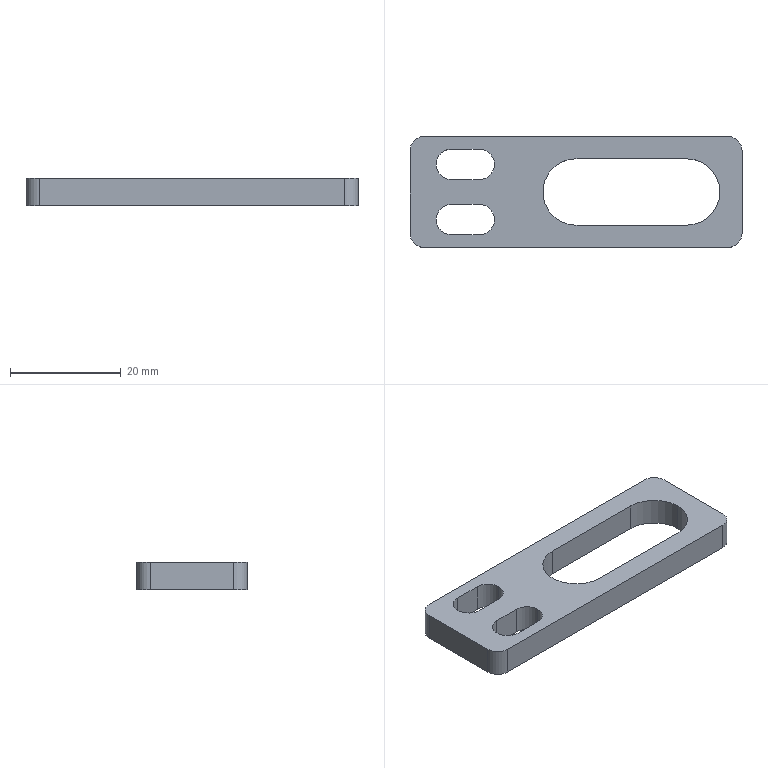Part | STEP file | KF-2212-050-005 | 1 solid | 25 faces | box 60 x 20 x 5 mm | volume 3695 mm3 | cylinder 13 | plane 12 | commonest cylinder face diameters 5.5 x6 5 x4 12 x3
STEP:
#1=CARTESIAN_POINT('',(-14.75,5.,-5.));
#2=VERTEX_POINT('',#1);
#3=CARTESIAN_POINT('',(-17.5,7.75,-5.));
#4=VERTEX_POINT('',#3);
#5=CARTESIAN_POINT('',(-17.5,5.,-5.));
#6=DIRECTION('',(0.,0.,1.));
#7=DIRECTION('',(1.,0.,0.));
#8=AXIS2_PLACEMENT_3D('',#5,#6,#7);
#9=CIRCLE('',#8,2.75);
#10=EDGE_CURVE('',#2,#4,#9,.T.);
#11=ORIENTED_EDGE('',*,*,#10,.F.);
#12=CARTESIAN_POINT('',(-14.75,5.,0.));
#13=VERTEX_POINT('',#12);
#14=CARTESIAN_POINT('',(-14.75,5.,-10.));
#15=DIRECTION('',(0.,0.,1.));
#16=VECTOR('',#15,1000.);
#17=LINE('',#14,#16);
#18=EDGE_CURVE('',#2,#13,#17,.T.);
#19=ORIENTED_EDGE('',*,*,#18,.T.);
#20=CARTESIAN_POINT('',(-17.5,7.75,0.));
#21=VERTEX_POINT('',#20);
#22=CARTESIAN_POINT('',(-17.5,5.,0.));
#23=DIRECTION('',(0.,0.,1.));
#24=DIRECTION('',(1.,0.,0.));
#25=AXIS2_PLACEMENT_3D('',#22,#23,#24);
#26=CIRCLE('',#25,2.75);
#27=EDGE_CURVE('',#13,#21,#26,.T.);
#28=ORIENTED_EDGE('',*,*,#27,.T.);
#29=CARTESIAN_POINT('',(-17.5,7.75,-10.));
#30=DIRECTION('',(0.,0.,1.));
#31=VECTOR('',#30,1000.);
#32=LINE('',#29,#31);
#33=EDGE_CURVE('',#4,#21,#32,.T.);
#34=ORIENTED_EDGE('',*,*,#33,.F.);
#35=EDGE_LOOP('',(#11,#19,#28,#34));
#36=FACE_OUTER_BOUND('',#35,.T.);
#37=CARTESIAN_POINT('',(-17.5,5.,-10.));
#38=DIRECTION('',(0.,0.,1.));
#39=DIRECTION('',(1.,0.,0.));
#40=AXIS2_PLACEMENT_3D('',#37,#38,#39);
#41=CYLINDRICAL_SURFACE('',#40,2.75);
#42=ADVANCED_FACE('',(#36),#41,.F.);
#43=CARTESIAN_POINT('',(-14.75,-5.,-5.));
#44=VERTEX_POINT('',#43);
#45=CARTESIAN_POINT('',(-17.5,-2.25,-5.));
#46=VERTEX_POINT('',#45);
#47=CARTESIAN_POINT('',(-17.5,-5.,-5.));
#48=DIRECTION('',(0.,0.,1.));
#49=DIRECTION('',(1.,0.,0.));
#50=AXIS2_PLACEMENT_3D('',#47,#48,#49);
#51=CIRCLE('',#50,2.75);
#52=EDGE_CURVE('',#44,#46,#51,.T.);
#53=ORIENTED_EDGE('',*,*,#52,.F.);
#54=CARTESIAN_POINT('',(-14.75,-5.,0.));
#55=VERTEX_POINT('',#54);
#56=CARTESIAN_POINT('',(-14.75,-5.,-10.));
#57=DIRECTION('',(0.,0.,1.));
#58=VECTOR('',#57,1000.);
#59=LINE('',#56,#58);
#60=EDGE_CURVE('',#44,#55,#59,.T.);
#61=ORIENTED_EDGE('',*,*,#60,.T.);
#62=CARTESIAN_POINT('',(-17.5,-2.25,0.));
#63=VERTEX_POINT('',#62);
#64=CARTESIAN_POINT('',(-17.5,-5.,0.));
#65=DIRECTION('',(0.,0.,1.));
#66=DIRECTION('',(1.,0.,0.));
#67=AXIS2_PLACEMENT_3D('',#64,#65,#66);
#68=CIRCLE('',#67,2.75);
#69=EDGE_CURVE('',#55,#63,#68,.T.);
#70=ORIENTED_EDGE('',*,*,#69,.T.);
#71=CARTESIAN_POINT('',(-17.5,-2.25,-10.));
#72=DIRECTION('',(0.,0.,1.));
#73=VECTOR('',#72,1000.);
#74=LINE('',#71,#73);
#75=EDGE_CURVE('',#46,#63,#74,.T.);
#76=ORIENTED_EDGE('',*,*,#75,.F.);
#77=EDGE_LOOP('',(#53,#61,#70,#76));
#78=FACE_OUTER_BOUND('',#77,.T.);
#79=CARTESIAN_POINT('',(-17.5,-5.,-10.));
#80=DIRECTION('',(0.,0.,1.));
#81=DIRECTION('',(1.,0.,0.));
#82=AXIS2_PLACEMENT_3D('',#79,#80,#81);
#83=CYLINDRICAL_SURFACE('',#82,2.75);
#84=ADVANCED_FACE('',(#78),#83,.F.);
#85=CARTESIAN_POINT('',(26.,0.,-5.));
#86=VERTEX_POINT('',#85);
#87=CARTESIAN_POINT('',(20.,6.,-5.));
#88=VERTEX_POINT('',#87);
#89=CARTESIAN_POINT('',(20.,0.,-5.));
#90=DIRECTION('',(0.,0.,1.));
#91=DIRECTION('',(1.,0.,0.));
#92=AXIS2_PLACEMENT_3D('',#89,#90,#91);
#93=CIRCLE('',#92,6.);
#94=EDGE_CURVE('',#86,#88,#93,.T.);
#95=ORIENTED_EDGE('',*,*,#94,.F.);
#96=CARTESIAN_POINT('',(26.,0.,0.));
#97=VERTEX_POINT('',#96);
#98=CARTESIAN_POINT('',(26.,0.,-5.));
#99=DIRECTION('',(0.,0.,1.));
#100=VECTOR('',#99,1000.);
#101=LINE('',#98,#100);
#102=EDGE_CURVE('',#86,#97,#101,.T.);
#103=ORIENTED_EDGE('',*,*,#102,.T.);
#104=CARTESIAN_POINT('',(20.,6.,0.));
#105=VERTEX_POINT('',#104);
#106=CARTESIAN_POINT('',(20.,0.,0.));
#107=DIRECTION('',(0.,0.,1.));
#108=DIRECTION('',(1.,0.,0.));
#109=AXIS2_PLACEMENT_3D('',#106,#107,#108);
#110=CIRCLE('',#109,6.);
#111=EDGE_CURVE('',#97,#105,#110,.T.);
#112=ORIENTED_EDGE('',*,*,#111,.T.);
#113=CARTESIAN_POINT('',(20.,6.,-5.));
#114=DIRECTION('',(0.,0.,1.));
#115=VECTOR('',#114,1000.);
#116=LINE('',#113,#115);
#117=EDGE_CURVE('',#88,#105,#116,.T.);
#118=ORIENTED_EDGE('',*,*,#117,.F.);
#119=EDGE_LOOP('',(#95,#103,#112,#118));
#120=FACE_OUTER_BOUND('',#119,.T.);
#121=CARTESIAN_POINT('',(20.,0.,-5.));
#122=DIRECTION('',(0.,0.,1.));
#123=DIRECTION('',(1.,0.,0.));
#124=AXIS2_PLACEMENT_3D('',#121,#122,#123);
#125=CYLINDRICAL_SURFACE('',#124,6.);
#126=ADVANCED_FACE('',(#120),#125,.F.);
#127=CARTESIAN_POINT('',(30.,-7.5,0.));
#128=VERTEX_POINT('',#127);
#129=CARTESIAN_POINT('',(30.,7.5,0.));
#130=VERTEX_POINT('',#129);
#131=CARTESIAN_POINT('',(30.,10.,0.));
#132=DIRECTION('',(0.,1.,0.));
#133=VECTOR('',#132,1000.);
#134=LINE('',#131,#133);
#135=EDGE_CURVE('',#128,#130,#134,.T.);
#136=ORIENTED_EDGE('',*,*,#135,.F.);
#137=CARTESIAN_POINT('',(30.,-7.5,-5.));
#138=VERTEX_POINT('',#137);
#139=CARTESIAN_POINT('',(30.,-7.5,-5.));
#140=DIRECTION('',(0.,0.,-1.));
#141=VECTOR('',#140,1000.);
#142=LINE('',#139,#141);
#143=EDGE_CURVE('',#128,#138,#142,.T.);
#144=ORIENTED_EDGE('',*,*,#143,.T.);
#145=CARTESIAN_POINT('',(30.,7.5,-5.));
#146=VERTEX_POINT('',#145);
#147=CARTESIAN_POINT('',(30.,10.,-5.));
#148=DIRECTION('',(0.,1.,0.));
#149=VECTOR('',#148,1000.);
#150=LINE('',#147,#149);
#151=EDGE_CURVE('',#138,#146,#150,.T.);
#152=ORIENTED_EDGE('',*,*,#151,.T.);
#153=CARTESIAN_POINT('',(30.,7.5,-5.));
#154=DIRECTION('',(0.,0.,1.));
#155=VECTOR('',#154,1000.);
#156=LINE('',#153,#155);
#157=EDGE_CURVE('',#146,#130,#156,.T.);
#158=ORIENTED_EDGE('',*,*,#157,.T.);
#159=EDGE_LOOP('',(#136,#144,#152,#158));
#160=FACE_OUTER_BOUND('',#159,.T.);
#161=CARTESIAN_POINT('',(30.,10.,-5.));
#162=DIRECTION('',(1.,0.,0.));
#163=DIRECTION('',(0.,0.,-1.));
#164=AXIS2_PLACEMENT_3D('',#161,#162,#163);
#165=PLANE('',#164);
#166=ADVANCED_FACE('',(#160),#165,.T.);
#167=CARTESIAN_POINT('',(-27.5,-10.,0.));
#168=VERTEX_POINT('',#167);
#169=CARTESIAN_POINT('',(27.5,-10.,0.));
#170=VERTEX_POINT('',#169);
#171=CARTESIAN_POINT('',(-30.,-10.,0.));
#172=DIRECTION('',(1.,0.,0.));
#173=VECTOR('',#172,1000.);
#174=LINE('',#171,#173);
#175=EDGE_CURVE('',#168,#170,#174,.T.);
#176=ORIENTED_EDGE('',*,*,#175,.F.);
#177=CARTESIAN_POINT('',(-27.5,-10.,-5.));
#178=VERTEX_POINT('',#177);
#179=CARTESIAN_POINT('',(-27.5,-10.,-5.));
#180=DIRECTION('',(0.,0.,-1.));
#181=VECTOR('',#180,1000.);
#182=LINE('',#179,#181);
#183=EDGE_CURVE('',#168,#178,#182,.T.);
#184=ORIENTED_EDGE('',*,*,#183,.T.);
#185=CARTESIAN_POINT('',(27.5,-10.,-5.));
#186=VERTEX_POINT('',#185);
#187=CARTESIAN_POINT('',(-30.,-10.,-5.));
#188=DIRECTION('',(1.,0.,0.));
#189=VECTOR('',#188,1000.);
#190=LINE('',#187,#189);
#191=EDGE_CURVE('',#178,#186,#190,.T.);
#192=ORIENTED_EDGE('',*,*,#191,.T.);
#193=CARTESIAN_POINT('',(27.5,-10.,-5.));
#194=DIRECTION('',(0.,0.,1.));
#195=VECTOR('',#194,1000.);
#196=LINE('',#193,#195);
#197=EDGE_CURVE('',#186,#170,#196,.T.);
#198=ORIENTED_EDGE('',*,*,#197,.T.);
#199=EDGE_LOOP('',(#176,#184,#192,#198));
#200=FACE_OUTER_BOUND('',#199,.T.);
#201=CARTESIAN_POINT('',(-30.,-10.,-5.));
#202=DIRECTION('',(0.,-1.,0.));
#203=DIRECTION('',(1.,0.,0.));
#204=AXIS2_PLACEMENT_3D('',#201,#202,#203);
#205=PLANE('',#204);
#206=ADVANCED_FACE('',(#200),#205,.T.);
#207=CARTESIAN_POINT('',(-30.,7.5,-5.));
#208=VERTEX_POINT('',#207);
#209=CARTESIAN_POINT('',(-30.,-7.5,-5.));
#210=VERTEX_POINT('',#209);
#211=CARTESIAN_POINT('',(-30.,10.,-5.));
#212=DIRECTION('',(0.,-1.,0.));
#213=VECTOR('',#212,1000.);
#214=LINE('',#211,#213);
#215=EDGE_CURVE('',#208,#210,#214,.T.);
#216=ORIENTED_EDGE('',*,*,#215,.T.);
#217=CARTESIAN_POINT('',(-30.,-7.5,0.));
#218=VERTEX_POINT('',#217);
#219=CARTESIAN_POINT('',(-30.,-7.5,-5.));
#220=DIRECTION('',(0.,0.,1.));
#221=VECTOR('',#220,1000.);
#222=LINE('',#219,#221);
#223=EDGE_CURVE('',#210,#218,#222,.T.);
#224=ORIENTED_EDGE('',*,*,#223,.T.);
#225=CARTESIAN_POINT('',(-30.,7.5,0.));
#226=VERTEX_POINT('',#225);
#227=CARTESIAN_POINT('',(-30.,10.,0.));
#228=DIRECTION('',(0.,-1.,0.));
#229=VECTOR('',#228,1000.);
#230=LINE('',#227,#229);
#231=EDGE_CURVE('',#226,#218,#230,.T.);
#232=ORIENTED_EDGE('',*,*,#231,.F.);
#233=CARTESIAN_POINT('',(-30.,7.5,-5.));
#234=DIRECTION('',(0.,0.,-1.));
#235=VECTOR('',#234,1000.);
#236=LINE('',#233,#235);
#237=EDGE_CURVE('',#226,#208,#236,.T.);
#238=ORIENTED_EDGE('',*,*,#237,.T.);
#239=EDGE_LOOP('',(#216,#224,#232,#238));
#240=FACE_OUTER_BOUND('',#239,.T.);
#241=CARTESIAN_POINT('',(-30.,10.,-5.));
#242=DIRECTION('',(-1.,0.,0.));
#243=DIRECTION('',(0.,0.,1.));
#244=AXIS2_PLACEMENT_3D('',#241,#242,#243);
#245=PLANE('',#244);
#246=ADVANCED_FACE('',(#240),#245,.T.);
#247=CARTESIAN_POINT('',(27.5,10.,-5.));
#248=VERTEX_POINT('',#247);
#249=CARTESIAN_POINT('',(-27.5,10.,-5.));
#250=VERTEX_POINT('',#249);
#251=CARTESIAN_POINT('',(-30.,10.,-5.));
#252=DIRECTION('',(-1.,0.,0.));
#253=VECTOR('',#252,1000.);
#254=LINE('',#251,#253);
#255=EDGE_CURVE('',#248,#250,#254,.T.);
#256=ORIENTED_EDGE('',*,*,#255,.T.);
#257=CARTESIAN_POINT('',(-27.5,10.,0.));
#258=VERTEX_POINT('',#257);
#259=CARTESIAN_POINT('',(-27.5,10.,-5.));
#260=DIRECTION('',(0.,0.,1.));
#261=VECTOR('',#260,1000.);
#262=LINE('',#259,#261);
#263=EDGE_CURVE('',#250,#258,#262,.T.);
#264=ORIENTED_EDGE('',*,*,#263,.T.);
#265=CARTESIAN_POINT('',(27.5,10.,0.));
#266=VERTEX_POINT('',#265);
#267=CARTESIAN_POINT('',(-30.,10.,0.));
#268=DIRECTION('',(-1.,0.,0.));
#269=VECTOR('',#268,1000.);
#270=LINE('',#267,#269);
#271=EDGE_CURVE('',#266,#258,#270,.T.);
#272=ORIENTED_EDGE('',*,*,#271,.F.);
#273=CARTESIAN_POINT('',(27.5,10.,-5.));
#274=DIRECTION('',(0.,0.,-1.));
#275=VECTOR('',#274,1000.);
#276=LINE('',#273,#275);
#277=EDGE_CURVE('',#266,#248,#276,.T.);
#278=ORIENTED_EDGE('',*,*,#277,.T.);
#279=EDGE_LOOP('',(#256,#264,#272,#278));
#280=FACE_OUTER_BOUND('',#279,.T.);
#281=CARTESIAN_POINT('',(-30.,10.,-5.));
#282=DIRECTION('',(0.,1.,0.));
#283=DIRECTION('',(-1.,0.,0.));
#284=AXIS2_PLACEMENT_3D('',#281,#282,#283);
#285=PLANE('',#284);
#286=ADVANCED_FACE('',(#280),#285,.T.);
#287=CARTESIAN_POINT('',(-22.5,7.75,-5.));
#288=VERTEX_POINT('',#287);
#289=CARTESIAN_POINT('',(0.,7.75,-5.));
#290=DIRECTION('',(-1.,0.,0.));
#291=VECTOR('',#290,1000.);
#292=LINE('',#289,#291);
#293=EDGE_CURVE('',#4,#288,#292,.T.);
#294=ORIENTED_EDGE('',*,*,#293,.T.);
#295=CARTESIAN_POINT('',(-22.5,2.25,-5.));
#296=VERTEX_POINT('',#295);
#297=CARTESIAN_POINT('',(-22.5,5.,-5.));
#298=DIRECTION('',(0.,0.,1.));
#299=DIRECTION('',(1.,0.,0.));
#300=AXIS2_PLACEMENT_3D('',#297,#298,#299);
#301=CIRCLE('',#300,2.75);
#302=EDGE_CURVE('',#288,#296,#301,.T.);
#303=ORIENTED_EDGE('',*,*,#302,.T.);
#304=CARTESIAN_POINT('',(-17.5,2.25,-5.));
#305=VERTEX_POINT('',#304);
#306=CARTESIAN_POINT('',(0.,2.25,-5.));
#307=DIRECTION('',(1.,0.,0.));
#308=VECTOR('',#307,1000.);
#309=LINE('',#306,#308);
#310=EDGE_CURVE('',#296,#305,#309,.T.);
#311=ORIENTED_EDGE('',*,*,#310,.T.);
#312=CARTESIAN_POINT('',(-17.5,5.,-5.));
#313=DIRECTION('',(0.,0.,1.));
#314=DIRECTION('',(1.,0.,0.));
#315=AXIS2_PLACEMENT_3D('',#312,#313,#314);
#316=CIRCLE('',#315,2.75);
#317=EDGE_CURVE('',#305,#2,#316,.T.);
#318=ORIENTED_EDGE('',*,*,#317,.T.);
#319=ORIENTED_EDGE('',*,*,#10,.T.);
#320=EDGE_LOOP('',(#294,#303,#311,#318,#319));
#321=FACE_BOUND('',#320,.T.);
#322=CARTESIAN_POINT('',(-22.5,-2.25,-5.));
#323=VERTEX_POINT('',#322);
#324=CARTESIAN_POINT('',(0.,-2.25,-5.));
#325=DIRECTION('',(-1.,0.,0.));
#326=VECTOR('',#325,1000.);
#327=LINE('',#324,#326);
#328=EDGE_CURVE('',#46,#323,#327,.T.);
#329=ORIENTED_EDGE('',*,*,#328,.T.);
#330=CARTESIAN_POINT('',(-22.5,-7.75,-5.));
#331=VERTEX_POINT('',#330);
#332=CARTESIAN_POINT('',(-22.5,-5.,-5.));
#333=DIRECTION('',(0.,0.,1.));
#334=DIRECTION('',(1.,0.,0.));
#335=AXIS2_PLACEMENT_3D('',#332,#333,#334);
#336=CIRCLE('',#335,2.75);
#337=EDGE_CURVE('',#323,#331,#336,.T.);
#338=ORIENTED_EDGE('',*,*,#337,.T.);
#339=CARTESIAN_POINT('',(-17.5,-7.75,-5.));
#340=VERTEX_POINT('',#339);
#341=CARTESIAN_POINT('',(0.,-7.75,-5.));
#342=DIRECTION('',(1.,0.,0.));
#343=VECTOR('',#342,1000.);
#344=LINE('',#341,#343);
#345=EDGE_CURVE('',#331,#340,#344,.T.);
#346=ORIENTED_EDGE('',*,*,#345,.T.);
#347=CARTESIAN_POINT('',(-17.5,-5.,-5.));
#348=DIRECTION('',(0.,0.,1.));
#349=DIRECTION('',(1.,0.,0.));
#350=AXIS2_PLACEMENT_3D('',#347,#348,#349);
#351=CIRCLE('',#350,2.75);
#352=EDGE_CURVE('',#340,#44,#351,.T.);
#353=ORIENTED_EDGE('',*,*,#352,.T.);
#354=ORIENTED_EDGE('',*,*,#52,.T.);
#355=EDGE_LOOP('',(#329,#338,#346,#353,#354));
#356=FACE_BOUND('',#355,.T.);
#357=CARTESIAN_POINT('',(0.,6.,-5.));
#358=VERTEX_POINT('',#357);
#359=CARTESIAN_POINT('',(0.,6.,-5.));
#360=DIRECTION('',(-1.,0.,0.));
#361=VECTOR('',#360,1000.);
#362=LINE('',#359,#361);
#363=EDGE_CURVE('',#88,#358,#362,.T.);
#364=ORIENTED_EDGE('',*,*,#363,.T.);
#365=CARTESIAN_POINT('',(0.,-6.,-5.));
#366=VERTEX_POINT('',#365);
#367=CARTESIAN_POINT('',(0.,0.,-5.));
#368=DIRECTION('',(0.,0.,1.));
#369=DIRECTION('',(1.,0.,0.));
#370=AXIS2_PLACEMENT_3D('',#367,#368,#369);
#371=CIRCLE('',#370,6.);
#372=EDGE_CURVE('',#358,#366,#371,.T.);
#373=ORIENTED_EDGE('',*,*,#372,.T.);
#374=CARTESIAN_POINT('',(20.,-6.,-5.));
#375=VERTEX_POINT('',#374);
#376=CARTESIAN_POINT('',(0.,-6.,-5.));
#377=DIRECTION('',(1.,0.,0.));
#378=VECTOR('',#377,1000.);
#379=LINE('',#376,#378);
#380=EDGE_CURVE('',#366,#375,#379,.T.);
#381=ORIENTED_EDGE('',*,*,#380,.T.);
#382=CARTESIAN_POINT('',(20.,0.,-5.));
#383=DIRECTION('',(0.,0.,1.));
#384=DIRECTION('',(1.,0.,0.));
#385=AXIS2_PLACEMENT_3D('',#382,#383,#384);
#386=CIRCLE('',#385,6.);
#387=EDGE_CURVE('',#375,#86,#386,.T.);
#388=ORIENTED_EDGE('',*,*,#387,.T.);
#389=ORIENTED_EDGE('',*,*,#94,.T.);
#390=EDGE_LOOP('',(#364,#373,#381,#388,#389));
#391=FACE_BOUND('',#390,.T.);
#392=ORIENTED_EDGE('',*,*,#191,.F.);
#393=CARTESIAN_POINT('',(-27.5,-7.5,-5.));
#394=DIRECTION('',(0.,0.,-1.));
#395=DIRECTION('',(1.,0.,0.));
#396=AXIS2_PLACEMENT_3D('',#393,#394,#395);
#397=CIRCLE('',#396,2.5);
#398=EDGE_CURVE('',#178,#210,#397,.T.);
#399=ORIENTED_EDGE('',*,*,#398,.T.);
#400=ORIENTED_EDGE('',*,*,#215,.F.);
#401=CARTESIAN_POINT('',(-27.5,7.5,-5.));
#402=DIRECTION('',(0.,0.,-1.));
#403=DIRECTION('',(1.,0.,0.));
#404=AXIS2_PLACEMENT_3D('',#401,#402,#403);
#405=CIRCLE('',#404,2.5);
#406=EDGE_CURVE('',#208,#250,#405,.T.);
#407=ORIENTED_EDGE('',*,*,#406,.T.);
#408=ORIENTED_EDGE('',*,*,#255,.F.);
#409=CARTESIAN_POINT('',(27.5,7.5,-5.));
#410=DIRECTION('',(0.,0.,-1.));
#411=DIRECTION('',(1.,0.,0.));
#412=AXIS2_PLACEMENT_3D('',#409,#410,#411);
#413=CIRCLE('',#412,2.5);
#414=EDGE_CURVE('',#248,#146,#413,.T.);
#415=ORIENTED_EDGE('',*,*,#414,.T.);
#416=ORIENTED_EDGE('',*,*,#151,.F.);
#417=CARTESIAN_POINT('',(27.5,-7.5,-5.));
#418=DIRECTION('',(0.,0.,-1.));
#419=DIRECTION('',(1.,0.,0.));
#420=AXIS2_PLACEMENT_3D('',#417,#418,#419);
#421=CIRCLE('',#420,2.5);
#422=EDGE_CURVE('',#138,#186,#421,.T.);
#423=ORIENTED_EDGE('',*,*,#422,.T.);
#424=EDGE_LOOP('',(#392,#399,#400,#407,#408,#415,#416,#423));
#425=FACE_OUTER_BOUND('',#424,.T.);
#426=CARTESIAN_POINT('',(0.,0.,-5.));
#427=DIRECTION('',(0.,0.,1.));
#428=DIRECTION('',(1.,0.,0.));
#429=AXIS2_PLACEMENT_3D('',#426,#427,#428);
#430=PLANE('',#429);
#431=ADVANCED_FACE('',(#321,#356,#391,#425),#430,.F.);
#432=CARTESIAN_POINT('',(-22.5,7.75,0.));
#433=VERTEX_POINT('',#432);
#434=CARTESIAN_POINT('',(-22.5,2.25,0.));
#435=VERTEX_POINT('',#434);
#436=CARTESIAN_POINT('',(-22.5,5.,0.));
#437=DIRECTION('',(0.,0.,1.));
#438=DIRECTION('',(1.,0.,0.));
#439=AXIS2_PLACEMENT_3D('',#436,#437,#438);
#440=CIRCLE('',#439,2.75);
#441=EDGE_CURVE('',#433,#435,#440,.T.);
#442=ORIENTED_EDGE('',*,*,#441,.F.);
#443=CARTESIAN_POINT('',(-22.5,7.75,0.));
#444=DIRECTION('',(-1.,0.,0.));
#445=VECTOR('',#444,1000.);
#446=LINE('',#443,#445);
#447=EDGE_CURVE('',#21,#433,#446,.T.);
#448=ORIENTED_EDGE('',*,*,#447,.F.);
#449=ORIENTED_EDGE('',*,*,#27,.F.);
#450=CARTESIAN_POINT('',(-17.5,2.25,0.));
#451=VERTEX_POINT('',#450);
#452=CARTESIAN_POINT('',(-17.5,5.,0.));
#453=DIRECTION('',(0.,0.,1.));
#454=DIRECTION('',(1.,0.,0.));
#455=AXIS2_PLACEMENT_3D('',#452,#453,#454);
#456=CIRCLE('',#455,2.75);
#457=EDGE_CURVE('',#451,#13,#456,.T.);
#458=ORIENTED_EDGE('',*,*,#457,.F.);
#459=CARTESIAN_POINT('',(-22.5,2.25,0.));
#460=DIRECTION('',(1.,0.,0.));
#461=VECTOR('',#460,1000.);
#462=LINE('',#459,#461);
#463=EDGE_CURVE('',#435,#451,#462,.T.);
#464=ORIENTED_EDGE('',*,*,#463,.F.);
#465=EDGE_LOOP('',(#442,#448,#449,#458,#464));
#466=FACE_BOUND('',#465,.T.);
#467=CARTESIAN_POINT('',(-22.5,-2.25,0.));
#468=VERTEX_POINT('',#467);
#469=CARTESIAN_POINT('',(-22.5,-7.75,0.));
#470=VERTEX_POINT('',#469);
#471=CARTESIAN_POINT('',(-22.5,-5.,0.));
#472=DIRECTION('',(0.,0.,1.));
#473=DIRECTION('',(1.,0.,0.));
#474=AXIS2_PLACEMENT_3D('',#471,#472,#473);
#475=CIRCLE('',#474,2.75);
#476=EDGE_CURVE('',#468,#470,#475,.T.);
#477=ORIENTED_EDGE('',*,*,#476,.F.);
#478=CARTESIAN_POINT('',(-22.5,-2.25,0.));
#479=DIRECTION('',(-1.,0.,0.));
#480=VECTOR('',#479,1000.);
#481=LINE('',#478,#480);
#482=EDGE_CURVE('',#63,#468,#481,.T.);
#483=ORIENTED_EDGE('',*,*,#482,.F.);
#484=ORIENTED_EDGE('',*,*,#69,.F.);
#485=CARTESIAN_POINT('',(-17.5,-7.75,0.));
#486=VERTEX_POINT('',#485);
#487=CARTESIAN_POINT('',(-17.5,-5.,0.));
#488=DIRECTION('',(0.,0.,1.));
#489=DIRECTION('',(1.,0.,0.));
#490=AXIS2_PLACEMENT_3D('',#487,#488,#489);
#491=CIRCLE('',#490,2.75);
#492=EDGE_CURVE('',#486,#55,#491,.T.);
#493=ORIENTED_EDGE('',*,*,#492,.F.);
#494=CARTESIAN_POINT('',(-22.5,-7.75,0.));
#495=DIRECTION('',(1.,0.,0.));
#496=VECTOR('',#495,1000.);
#497=LINE('',#494,#496);
#498=EDGE_CURVE('',#470,#486,#497,.T.);
#499=ORIENTED_EDGE('',*,*,#498,.F.);
#500=EDGE_LOOP('',(#477,#483,#484,#493,#499));
#501=FACE_BOUND('',#500,.T.);
#502=CARTESIAN_POINT('',(0.,6.,0.));
#503=VERTEX_POINT('',#502);
#504=CARTESIAN_POINT('',(0.,-6.,0.));
#505=VERTEX_POINT('',#504);
#506=CARTESIAN_POINT('',(0.,0.,0.));
#507=DIRECTION('',(0.,0.,1.));
#508=DIRECTION('',(1.,0.,0.));
#509=AXIS2_PLACEMENT_3D('',#506,#507,#508);
#510=CIRCLE('',#509,6.);
#511=EDGE_CURVE('',#503,#505,#510,.T.);
#512=ORIENTED_EDGE('',*,*,#511,.F.);
#513=CARTESIAN_POINT('',(0.,6.,0.));
#514=DIRECTION('',(-1.,0.,0.));
#515=VECTOR('',#514,1000.);
#516=LINE('',#513,#515);
#517=EDGE_CURVE('',#105,#503,#516,.T.);
#518=ORIENTED_EDGE('',*,*,#517,.F.);
#519=ORIENTED_EDGE('',*,*,#111,.F.);
#520=CARTESIAN_POINT('',(20.,-6.,0.));
#521=VERTEX_POINT('',#520);
#522=CARTESIAN_POINT('',(20.,0.,0.));
#523=DIRECTION('',(0.,0.,1.));
#524=DIRECTION('',(1.,0.,0.));
#525=AXIS2_PLACEMENT_3D('',#522,#523,#524);
#526=CIRCLE('',#525,6.);
#527=EDGE_CURVE('',#521,#97,#526,.T.);
#528=ORIENTED_EDGE('',*,*,#527,.F.);
#529=CARTESIAN_POINT('',(0.,-6.,0.));
#530=DIRECTION('',(1.,0.,0.));
#531=VECTOR('',#530,1000.);
#532=LINE('',#529,#531);
#533=EDGE_CURVE('',#505,#521,#532,.T.);
#534=ORIENTED_EDGE('',*,*,#533,.F.);
#535=EDGE_LOOP('',(#512,#518,#519,#528,#534));
#536=FACE_BOUND('',#535,.T.);
#537=ORIENTED_EDGE('',*,*,#231,.T.);
#538=CARTESIAN_POINT('',(-27.5,-7.5,0.));
#539=DIRECTION('',(0.,0.,1.));
#540=DIRECTION('',(1.,0.,0.));
#541=AXIS2_PLACEMENT_3D('',#538,#539,#540);
#542=CIRCLE('',#541,2.5);
#543=EDGE_CURVE('',#218,#168,#542,.T.);
#544=ORIENTED_EDGE('',*,*,#543,.T.);
#545=ORIENTED_EDGE('',*,*,#175,.T.);
#546=CARTESIAN_POINT('',(27.5,-7.5,0.));
#547=DIRECTION('',(0.,0.,1.));
#548=DIRECTION('',(1.,0.,0.));
#549=AXIS2_PLACEMENT_3D('',#546,#547,#548);
#550=CIRCLE('',#549,2.5);
#551=EDGE_CURVE('',#170,#128,#550,.T.);
#552=ORIENTED_EDGE('',*,*,#551,.T.);
#553=ORIENTED_EDGE('',*,*,#135,.T.);
#554=CARTESIAN_POINT('',(27.5,7.5,0.));
#555=DIRECTION('',(0.,0.,1.));
#556=DIRECTION('',(1.,0.,0.));
#557=AXIS2_PLACEMENT_3D('',#554,#555,#556);
#558=CIRCLE('',#557,2.5);
#559=EDGE_CURVE('',#130,#266,#558,.T.);
#560=ORIENTED_EDGE('',*,*,#559,.T.);
#561=ORIENTED_EDGE('',*,*,#271,.T.);
#562=CARTESIAN_POINT('',(-27.5,7.5,0.));
#563=DIRECTION('',(0.,0.,1.));
#564=DIRECTION('',(1.,0.,0.));
#565=AXIS2_PLACEMENT_3D('',#562,#563,#564);
#566=CIRCLE('',#565,2.5);
#567=EDGE_CURVE('',#258,#226,#566,.T.);
#568=ORIENTED_EDGE('',*,*,#567,.T.);
#569=EDGE_LOOP('',(#537,#544,#545,#552,#553,#560,#561,#568));
#570=FACE_OUTER_BOUND('',#569,.T.);
#571=CARTESIAN_POINT('',(0.,0.,0.));
#572=DIRECTION('',(0.,0.,1.));
#573=DIRECTION('',(1.,0.,0.));
#574=AXIS2_PLACEMENT_3D('',#571,#572,#573);
#575=PLANE('',#574);
#576=ADVANCED_FACE('',(#466,#501,#536,#570),#575,.T.);
#577=ORIENTED_EDGE('',*,*,#511,.T.);
#578=CARTESIAN_POINT('',(0.,-6.,-5.));
#579=DIRECTION('',(0.,0.,1.));
#580=VECTOR('',#579,1000.);
#581=LINE('',#578,#580);
#582=EDGE_CURVE('',#366,#505,#581,.T.);
#583=ORIENTED_EDGE('',*,*,#582,.F.);
#584=ORIENTED_EDGE('',*,*,#372,.F.);
#585=CARTESIAN_POINT('',(0.,6.,-5.));
#586=DIRECTION('',(0.,0.,1.));
#587=VECTOR('',#586,1000.);
#588=LINE('',#585,#587);
#589=EDGE_CURVE('',#358,#503,#588,.T.);
#590=ORIENTED_EDGE('',*,*,#589,.T.);
#591=EDGE_LOOP('',(#577,#583,#584,#590));
#592=FACE_OUTER_BOUND('',#591,.T.);
#593=CARTESIAN_POINT('',(0.,0.,-5.));
#594=DIRECTION('',(0.,0.,1.));
#595=DIRECTION('',(1.,0.,0.));
#596=AXIS2_PLACEMENT_3D('',#593,#594,#595);
#597=CYLINDRICAL_SURFACE('',#596,6.);
#598=ADVANCED_FACE('',(#592),#597,.F.);
#599=ORIENTED_EDGE('',*,*,#517,.T.);
#600=ORIENTED_EDGE('',*,*,#589,.F.);
#601=ORIENTED_EDGE('',*,*,#363,.F.);
#602=ORIENTED_EDGE('',*,*,#117,.T.);
#603=EDGE_LOOP('',(#599,#600,#601,#602));
#604=FACE_OUTER_BOUND('',#603,.T.);
#605=CARTESIAN_POINT('',(0.,6.,-5.));
#606=DIRECTION('',(0.,1.,0.));
#607=DIRECTION('',(-1.,0.,0.));
#608=AXIS2_PLACEMENT_3D('',#605,#606,#607);
#609=PLANE('',#608);
#610=ADVANCED_FACE('',(#604),#609,.F.);
#611=ORIENTED_EDGE('',*,*,#102,.F.);
#612=ORIENTED_EDGE('',*,*,#387,.F.);
#613=CARTESIAN_POINT('',(20.,-6.,-5.));
#614=DIRECTION('',(0.,0.,1.));
#615=VECTOR('',#614,1000.);
#616=LINE('',#613,#615);
#617=EDGE_CURVE('',#375,#521,#616,.T.);
#618=ORIENTED_EDGE('',*,*,#617,.T.);
#619=ORIENTED_EDGE('',*,*,#527,.T.);
#620=EDGE_LOOP('',(#611,#612,#618,#619));
#621=FACE_OUTER_BOUND('',#620,.T.);
#622=CARTESIAN_POINT('',(20.,0.,-5.));
#623=DIRECTION('',(0.,0.,1.));
#624=DIRECTION('',(1.,0.,0.));
#625=AXIS2_PLACEMENT_3D('',#622,#623,#624);
#626=CYLINDRICAL_SURFACE('',#625,6.);
#627=ADVANCED_FACE('',(#621),#626,.F.);
#628=ORIENTED_EDGE('',*,*,#533,.T.);
#629=ORIENTED_EDGE('',*,*,#617,.F.);
#630=ORIENTED_EDGE('',*,*,#380,.F.);
#631=ORIENTED_EDGE('',*,*,#582,.T.);
#632=EDGE_LOOP('',(#628,#629,#630,#631));
#633=FACE_OUTER_BOUND('',#632,.T.);
#634=CARTESIAN_POINT('',(0.,-6.,-5.));
#635=DIRECTION('',(0.,-1.,0.));
#636=DIRECTION('',(1.,0.,0.));
#637=AXIS2_PLACEMENT_3D('',#634,#635,#636);
#638=PLANE('',#637);
#639=ADVANCED_FACE('',(#633),#638,.F.);
#640=ORIENTED_EDGE('',*,*,#398,.F.);
#641=ORIENTED_EDGE('',*,*,#183,.F.);
#642=ORIENTED_EDGE('',*,*,#543,.F.);
#643=ORIENTED_EDGE('',*,*,#223,.F.);
#644=EDGE_LOOP('',(#640,#641,#642,#643));
#645=FACE_OUTER_BOUND('',#644,.T.);
#646=CARTESIAN_POINT('',(-27.5,-7.5,-5.));
#647=DIRECTION('',(0.,0.,1.));
#648=DIRECTION('',(1.,0.,0.));
#649=AXIS2_PLACEMENT_3D('',#646,#647,#648);
#650=CYLINDRICAL_SURFACE('',#649,2.5);
#651=ADVANCED_FACE('',(#645),#650,.T.);
#652=ORIENTED_EDGE('',*,*,#406,.F.);
#653=ORIENTED_EDGE('',*,*,#237,.F.);
#654=ORIENTED_EDGE('',*,*,#567,.F.);
#655=ORIENTED_EDGE('',*,*,#263,.F.);
#656=EDGE_LOOP('',(#652,#653,#654,#655));
#657=FACE_OUTER_BOUND('',#656,.T.);
#658=CARTESIAN_POINT('',(-27.5,7.5,-5.));
#659=DIRECTION('',(0.,0.,1.));
#660=DIRECTION('',(1.,0.,0.));
#661=AXIS2_PLACEMENT_3D('',#658,#659,#660);
#662=CYLINDRICAL_SURFACE('',#661,2.5);
#663=ADVANCED_FACE('',(#657),#662,.T.);
#664=ORIENTED_EDGE('',*,*,#422,.F.);
#665=ORIENTED_EDGE('',*,*,#143,.F.);
#666=ORIENTED_EDGE('',*,*,#551,.F.);
#667=ORIENTED_EDGE('',*,*,#197,.F.);
#668=EDGE_LOOP('',(#664,#665,#666,#667));
#669=FACE_OUTER_BOUND('',#668,.T.);
#670=CARTESIAN_POINT('',(27.5,-7.5,-5.));
#671=DIRECTION('',(0.,0.,1.));
#672=DIRECTION('',(1.,0.,0.));
#673=AXIS2_PLACEMENT_3D('',#670,#671,#672);
#674=CYLINDRICAL_SURFACE('',#673,2.5);
#675=ADVANCED_FACE('',(#669),#674,.T.);
#676=ORIENTED_EDGE('',*,*,#414,.F.);
#677=ORIENTED_EDGE('',*,*,#277,.F.);
#678=ORIENTED_EDGE('',*,*,#559,.F.);
#679=ORIENTED_EDGE('',*,*,#157,.F.);
#680=EDGE_LOOP('',(#676,#677,#678,#679));
#681=FACE_OUTER_BOUND('',#680,.T.);
#682=CARTESIAN_POINT('',(27.5,7.5,-5.));
#683=DIRECTION('',(0.,0.,1.));
#684=DIRECTION('',(1.,0.,0.));
#685=AXIS2_PLACEMENT_3D('',#682,#683,#684);
#686=CYLINDRICAL_SURFACE('',#685,2.5);
#687=ADVANCED_FACE('',(#681),#686,.T.);
#688=CARTESIAN_POINT('',(-22.5,-2.25,-10.));
#689=DIRECTION('',(0.,0.,1.));
#690=VECTOR('',#689,1000.);
#691=LINE('',#688,#690);
#692=EDGE_CURVE('',#323,#468,#691,.T.);
#693=ORIENTED_EDGE('',*,*,#692,.T.);
#694=ORIENTED_EDGE('',*,*,#476,.T.);
#695=CARTESIAN_POINT('',(-22.5,-7.75,-10.));
#696=DIRECTION('',(0.,0.,1.));
#697=VECTOR('',#696,1000.);
#698=LINE('',#695,#697);
#699=EDGE_CURVE('',#331,#470,#698,.T.);
#700=ORIENTED_EDGE('',*,*,#699,.F.);
#701=ORIENTED_EDGE('',*,*,#337,.F.);
#702=EDGE_LOOP('',(#693,#694,#700,#701));
#703=FACE_OUTER_BOUND('',#702,.T.);
#704=CARTESIAN_POINT('',(-22.5,-5.,-10.));
#705=DIRECTION('',(0.,0.,1.));
#706=DIRECTION('',(1.,0.,0.));
#707=AXIS2_PLACEMENT_3D('',#704,#705,#706);
#708=CYLINDRICAL_SURFACE('',#707,2.75);
#709=ADVANCED_FACE('',(#703),#708,.F.);
#710=ORIENTED_EDGE('',*,*,#75,.T.);
#711=ORIENTED_EDGE('',*,*,#482,.T.);
#712=ORIENTED_EDGE('',*,*,#692,.F.);
#713=ORIENTED_EDGE('',*,*,#328,.F.);
#714=EDGE_LOOP('',(#710,#711,#712,#713));
#715=FACE_OUTER_BOUND('',#714,.T.);
#716=CARTESIAN_POINT('',(-22.5,-2.25,-10.));
#717=DIRECTION('',(0.,1.,0.));
#718=DIRECTION('',(-1.,0.,0.));
#719=AXIS2_PLACEMENT_3D('',#716,#717,#718);
#720=PLANE('',#719);
#721=ADVANCED_FACE('',(#715),#720,.F.);
#722=ORIENTED_EDGE('',*,*,#60,.F.);
#723=ORIENTED_EDGE('',*,*,#352,.F.);
#724=CARTESIAN_POINT('',(-17.5,-7.75,-10.));
#725=DIRECTION('',(0.,0.,1.));
#726=VECTOR('',#725,1000.);
#727=LINE('',#724,#726);
#728=EDGE_CURVE('',#340,#486,#727,.T.);
#729=ORIENTED_EDGE('',*,*,#728,.T.);
#730=ORIENTED_EDGE('',*,*,#492,.T.);
#731=EDGE_LOOP('',(#722,#723,#729,#730));
#732=FACE_OUTER_BOUND('',#731,.T.);
#733=CARTESIAN_POINT('',(-17.5,-5.,-10.));
#734=DIRECTION('',(0.,0.,1.));
#735=DIRECTION('',(1.,0.,0.));
#736=AXIS2_PLACEMENT_3D('',#733,#734,#735);
#737=CYLINDRICAL_SURFACE('',#736,2.75);
#738=ADVANCED_FACE('',(#732),#737,.F.);
#739=ORIENTED_EDGE('',*,*,#699,.T.);
#740=ORIENTED_EDGE('',*,*,#498,.T.);
#741=ORIENTED_EDGE('',*,*,#728,.F.);
#742=ORIENTED_EDGE('',*,*,#345,.F.);
#743=EDGE_LOOP('',(#739,#740,#741,#742));
#744=FACE_OUTER_BOUND('',#743,.T.);
#745=CARTESIAN_POINT('',(-22.5,-7.75,-10.));
#746=DIRECTION('',(0.,-1.,0.));
#747=DIRECTION('',(1.,0.,0.));
#748=AXIS2_PLACEMENT_3D('',#745,#746,#747);
#749=PLANE('',#748);
#750=ADVANCED_FACE('',(#744),#749,.F.);
#751=CARTESIAN_POINT('',(-22.5,7.75,-10.));
#752=DIRECTION('',(0.,0.,1.));
#753=VECTOR('',#752,1000.);
#754=LINE('',#751,#753);
#755=EDGE_CURVE('',#288,#433,#754,.T.);
#756=ORIENTED_EDGE('',*,*,#755,.T.);
#757=ORIENTED_EDGE('',*,*,#441,.T.);
#758=CARTESIAN_POINT('',(-22.5,2.25,-10.));
#759=DIRECTION('',(0.,0.,1.));
#760=VECTOR('',#759,1000.);
#761=LINE('',#758,#760);
#762=EDGE_CURVE('',#296,#435,#761,.T.);
#763=ORIENTED_EDGE('',*,*,#762,.F.);
#764=ORIENTED_EDGE('',*,*,#302,.F.);
#765=EDGE_LOOP('',(#756,#757,#763,#764));
#766=FACE_OUTER_BOUND('',#765,.T.);
#767=CARTESIAN_POINT('',(-22.5,5.,-10.));
#768=DIRECTION('',(0.,0.,1.));
#769=DIRECTION('',(1.,0.,0.));
#770=AXIS2_PLACEMENT_3D('',#767,#768,#769);
#771=CYLINDRICAL_SURFACE('',#770,2.75);
#772=ADVANCED_FACE('',(#766),#771,.F.);
#773=ORIENTED_EDGE('',*,*,#33,.T.);
#774=ORIENTED_EDGE('',*,*,#447,.T.);
#775=ORIENTED_EDGE('',*,*,#755,.F.);
#776=ORIENTED_EDGE('',*,*,#293,.F.);
#777=EDGE_LOOP('',(#773,#774,#775,#776));
#778=FACE_OUTER_BOUND('',#777,.T.);
#779=CARTESIAN_POINT('',(-22.5,7.75,-10.));
#780=DIRECTION('',(0.,1.,0.));
#781=DIRECTION('',(-1.,0.,0.));
#782=AXIS2_PLACEMENT_3D('',#779,#780,#781);
#783=PLANE('',#782);
#784=ADVANCED_FACE('',(#778),#783,.F.);
#785=ORIENTED_EDGE('',*,*,#18,.F.);
#786=ORIENTED_EDGE('',*,*,#317,.F.);
#787=CARTESIAN_POINT('',(-17.5,2.25,-10.));
#788=DIRECTION('',(0.,0.,1.));
#789=VECTOR('',#788,1000.);
#790=LINE('',#787,#789);
#791=EDGE_CURVE('',#305,#451,#790,.T.);
#792=ORIENTED_EDGE('',*,*,#791,.T.);
#793=ORIENTED_EDGE('',*,*,#457,.T.);
#794=EDGE_LOOP('',(#785,#786,#792,#793));
#795=FACE_OUTER_BOUND('',#794,.T.);
#796=CARTESIAN_POINT('',(-17.5,5.,-10.));
#797=DIRECTION('',(0.,0.,1.));
#798=DIRECTION('',(1.,0.,0.));
#799=AXIS2_PLACEMENT_3D('',#796,#797,#798);
#800=CYLINDRICAL_SURFACE('',#799,2.75);
#801=ADVANCED_FACE('',(#795),#800,.F.);
#802=ORIENTED_EDGE('',*,*,#762,.T.);
#803=ORIENTED_EDGE('',*,*,#463,.T.);
#804=ORIENTED_EDGE('',*,*,#791,.F.);
#805=ORIENTED_EDGE('',*,*,#310,.F.);
#806=EDGE_LOOP('',(#802,#803,#804,#805));
#807=FACE_OUTER_BOUND('',#806,.T.);
#808=CARTESIAN_POINT('',(-22.5,2.25,-10.));
#809=DIRECTION('',(0.,-1.,0.));
#810=DIRECTION('',(1.,0.,0.));
#811=AXIS2_PLACEMENT_3D('',#808,#809,#810);
#812=PLANE('',#811);
#813=ADVANCED_FACE('',(#807),#812,.F.);
#814=CLOSED_SHELL('',(#42,#84,#126,#166,#206,#246,#286,#431,#576,#598,#610,#627,#639,#651,#663,#675,#687,#709,#721,#738,#750,#772,#784,#801,#813));
#815=MANIFOLD_SOLID_BREP('',#814);
#816=CARTESIAN_POINT('',(0.,0.,0.));
#817=DIRECTION('',(0.,0.,1.));
#818=DIRECTION('',(1.,0.,0.));
#819=AXIS2_PLACEMENT_3D('',#816,#817,#818);
#820=(LENGTH_UNIT()NAMED_UNIT(*)SI_UNIT(.MILLI.,.METRE.));
#821=UNCERTAINTY_MEASURE_WITH_UNIT(LENGTH_MEASURE(0.00001),#820,'','');
#822=(NAMED_UNIT(*)PLANE_ANGLE_UNIT()SI_UNIT($,.RADIAN.));
#823=(NAMED_UNIT(*)SI_UNIT($,.STERADIAN.)SOLID_ANGLE_UNIT());
#824=(GEOMETRIC_REPRESENTATION_CONTEXT(3)GLOBAL_UNCERTAINTY_ASSIGNED_CONTEXT((#821))GLOBAL_UNIT_ASSIGNED_CONTEXT((#820,#822,#823))REPRESENTATION_CONTEXT('',''));
#825=ADVANCED_BREP_SHAPE_REPRESENTATION('',(#815,#819),#824);